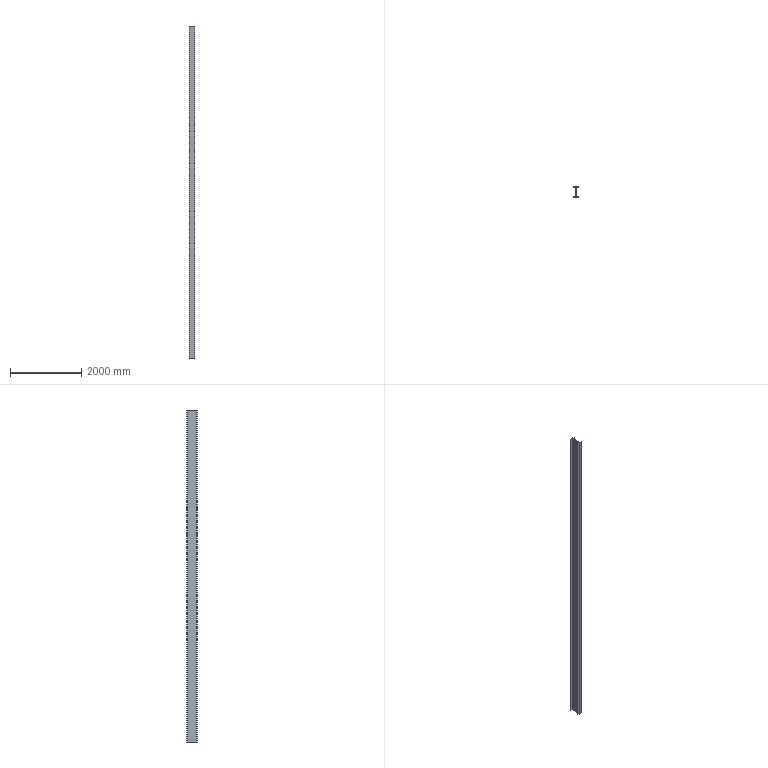Part | SolidWorks | features Extrusion 1 | 1 solid | 18 faces | box 150 x 300 x 9347 mm | volume 43725928 mm3 | plane 14 | cylinder 4 | commonest cylinder face diameters 26 x4
STEP:
#1=CARTESIAN_POINT('',(-75.,9.,0.));
#2=VERTEX_POINT('',#1);
#3=CARTESIAN_POINT('',(-75.,0.,0.));
#4=VERTEX_POINT('',#3);
#5=CARTESIAN_POINT('',(-75.,0.,0.));
#6=DIRECTION('',(0.,-1.,0.));
#7=VECTOR('',#6,1000.);
#8=LINE('',#5,#7);
#9=EDGE_CURVE('',#2,#4,#8,.T.);
#10=ORIENTED_EDGE('',*,*,#9,.T.);
#11=CARTESIAN_POINT('',(-75.,0.,9347.));
#12=VERTEX_POINT('',#11);
#13=CARTESIAN_POINT('',(-75.,0.,9347.));
#14=DIRECTION('',(0.,0.,-1.));
#15=VECTOR('',#14,1000.);
#16=LINE('',#13,#15);
#17=EDGE_CURVE('',#12,#4,#16,.T.);
#18=ORIENTED_EDGE('',*,*,#17,.F.);
#19=CARTESIAN_POINT('',(-75.,9.,9347.));
#20=VERTEX_POINT('',#19);
#21=CARTESIAN_POINT('',(-75.,0.,9347.));
#22=DIRECTION('',(0.,-1.,0.));
#23=VECTOR('',#22,1000.);
#24=LINE('',#21,#23);
#25=EDGE_CURVE('',#20,#12,#24,.T.);
#26=ORIENTED_EDGE('',*,*,#25,.F.);
#27=CARTESIAN_POINT('',(-75.,9.,9347.));
#28=DIRECTION('',(0.,0.,-1.));
#29=VECTOR('',#28,1000.);
#30=LINE('',#27,#29);
#31=EDGE_CURVE('',#20,#2,#30,.T.);
#32=ORIENTED_EDGE('',*,*,#31,.T.);
#33=EDGE_LOOP('',(#10,#18,#26,#32));
#34=FACE_OUTER_BOUND('',#33,.T.);
#35=CARTESIAN_POINT('',(-75.,0.,9347.));
#36=DIRECTION('',(1.,0.,0.));
#37=DIRECTION('',(0.,0.,-1.));
#38=AXIS2_PLACEMENT_3D('',#35,#36,#37);
#39=PLANE('',#38);
#40=ADVANCED_FACE('',(#34),#39,.F.);
#41=CARTESIAN_POINT('',(75.,0.,0.));
#42=VERTEX_POINT('',#41);
#43=CARTESIAN_POINT('',(75.,0.,0.));
#44=DIRECTION('',(1.,0.,0.));
#45=VECTOR('',#44,1000.);
#46=LINE('',#43,#45);
#47=EDGE_CURVE('',#4,#42,#46,.T.);
#48=ORIENTED_EDGE('',*,*,#47,.T.);
#49=CARTESIAN_POINT('',(75.,0.,9347.));
#50=VERTEX_POINT('',#49);
#51=CARTESIAN_POINT('',(75.,0.,9347.));
#52=DIRECTION('',(0.,0.,-1.));
#53=VECTOR('',#52,1000.);
#54=LINE('',#51,#53);
#55=EDGE_CURVE('',#50,#42,#54,.T.);
#56=ORIENTED_EDGE('',*,*,#55,.F.);
#57=CARTESIAN_POINT('',(75.,0.,9347.));
#58=DIRECTION('',(1.,0.,0.));
#59=VECTOR('',#58,1000.);
#60=LINE('',#57,#59);
#61=EDGE_CURVE('',#12,#50,#60,.T.);
#62=ORIENTED_EDGE('',*,*,#61,.F.);
#63=ORIENTED_EDGE('',*,*,#17,.T.);
#64=EDGE_LOOP('',(#48,#56,#62,#63));
#65=FACE_OUTER_BOUND('',#64,.T.);
#66=CARTESIAN_POINT('',(75.,0.,9347.));
#67=DIRECTION('',(0.,1.,0.));
#68=DIRECTION('',(-1.,0.,0.));
#69=AXIS2_PLACEMENT_3D('',#66,#67,#68);
#70=PLANE('',#69);
#71=ADVANCED_FACE('',(#65),#70,.F.);
#72=CARTESIAN_POINT('',(75.,9.,0.));
#73=VERTEX_POINT('',#72);
#74=CARTESIAN_POINT('',(75.,0.,0.));
#75=DIRECTION('',(0.,1.,0.));
#76=VECTOR('',#75,1000.);
#77=LINE('',#74,#76);
#78=EDGE_CURVE('',#42,#73,#77,.T.);
#79=ORIENTED_EDGE('',*,*,#78,.T.);
#80=CARTESIAN_POINT('',(75.,9.,9347.));
#81=VERTEX_POINT('',#80);
#82=CARTESIAN_POINT('',(75.,9.,9347.));
#83=DIRECTION('',(0.,0.,-1.));
#84=VECTOR('',#83,1000.);
#85=LINE('',#82,#84);
#86=EDGE_CURVE('',#81,#73,#85,.T.);
#87=ORIENTED_EDGE('',*,*,#86,.F.);
#88=CARTESIAN_POINT('',(75.,0.,9347.));
#89=DIRECTION('',(0.,1.,0.));
#90=VECTOR('',#89,1000.);
#91=LINE('',#88,#90);
#92=EDGE_CURVE('',#50,#81,#91,.T.);
#93=ORIENTED_EDGE('',*,*,#92,.F.);
#94=ORIENTED_EDGE('',*,*,#55,.T.);
#95=EDGE_LOOP('',(#79,#87,#93,#94));
#96=FACE_OUTER_BOUND('',#95,.T.);
#97=CARTESIAN_POINT('',(75.,0.,9347.));
#98=DIRECTION('',(-1.,0.,0.));
#99=DIRECTION('',(0.,0.,1.));
#100=AXIS2_PLACEMENT_3D('',#97,#98,#99);
#101=PLANE('',#100);
#102=ADVANCED_FACE('',(#96),#101,.F.);
#103=CARTESIAN_POINT('',(16.25,9.,0.));
#104=VERTEX_POINT('',#103);
#105=CARTESIAN_POINT('',(75.,9.,0.));
#106=DIRECTION('',(-1.,0.,0.));
#107=VECTOR('',#106,1000.);
#108=LINE('',#105,#107);
#109=EDGE_CURVE('',#73,#104,#108,.T.);
#110=ORIENTED_EDGE('',*,*,#109,.T.);
#111=CARTESIAN_POINT('',(16.25,9.,9347.));
#112=VERTEX_POINT('',#111);
#113=CARTESIAN_POINT('',(16.25,9.,9347.));
#114=DIRECTION('',(0.,0.,-1.));
#115=VECTOR('',#114,1000.);
#116=LINE('',#113,#115);
#117=EDGE_CURVE('',#112,#104,#116,.T.);
#118=ORIENTED_EDGE('',*,*,#117,.F.);
#119=CARTESIAN_POINT('',(75.,9.,9347.));
#120=DIRECTION('',(-1.,0.,0.));
#121=VECTOR('',#120,1000.);
#122=LINE('',#119,#121);
#123=EDGE_CURVE('',#81,#112,#122,.T.);
#124=ORIENTED_EDGE('',*,*,#123,.F.);
#125=ORIENTED_EDGE('',*,*,#86,.T.);
#126=EDGE_LOOP('',(#110,#118,#124,#125));
#127=FACE_OUTER_BOUND('',#126,.T.);
#128=CARTESIAN_POINT('',(75.,9.,9347.));
#129=DIRECTION('',(0.,-1.,0.));
#130=DIRECTION('',(1.,0.,0.));
#131=AXIS2_PLACEMENT_3D('',#128,#129,#130);
#132=PLANE('',#131);
#133=ADVANCED_FACE('',(#127),#132,.F.);
#134=CARTESIAN_POINT('',(3.25,22.,0.));
#135=VERTEX_POINT('',#134);
#136=CARTESIAN_POINT('',(16.25,22.,0.));
#137=DIRECTION('',(0.,0.,-1.));
#138=DIRECTION('',(-1.,0.,0.));
#139=AXIS2_PLACEMENT_3D('',#136,#137,#138);
#140=CIRCLE('',#139,13.);
#141=EDGE_CURVE('',#104,#135,#140,.T.);
#142=ORIENTED_EDGE('',*,*,#141,.T.);
#143=CARTESIAN_POINT('',(3.25,22.,9347.));
#144=VERTEX_POINT('',#143);
#145=CARTESIAN_POINT('',(3.25,22.,9347.));
#146=DIRECTION('',(0.,0.,-1.));
#147=VECTOR('',#146,1000.);
#148=LINE('',#145,#147);
#149=EDGE_CURVE('',#144,#135,#148,.T.);
#150=ORIENTED_EDGE('',*,*,#149,.F.);
#151=CARTESIAN_POINT('',(16.25,22.,9347.));
#152=DIRECTION('',(0.,0.,-1.));
#153=DIRECTION('',(-1.,0.,0.));
#154=AXIS2_PLACEMENT_3D('',#151,#152,#153);
#155=CIRCLE('',#154,13.);
#156=EDGE_CURVE('',#112,#144,#155,.T.);
#157=ORIENTED_EDGE('',*,*,#156,.F.);
#158=ORIENTED_EDGE('',*,*,#117,.T.);
#159=EDGE_LOOP('',(#142,#150,#157,#158));
#160=FACE_OUTER_BOUND('',#159,.T.);
#161=CARTESIAN_POINT('',(16.25,22.,9347.));
#162=DIRECTION('',(0.,0.,-1.));
#163=DIRECTION('',(-1.,0.,0.));
#164=AXIS2_PLACEMENT_3D('',#161,#162,#163);
#165=CYLINDRICAL_SURFACE('',#164,13.);
#166=ADVANCED_FACE('',(#160),#165,.F.);
#167=CARTESIAN_POINT('',(3.25,278.,0.));
#168=VERTEX_POINT('',#167);
#169=CARTESIAN_POINT('',(3.25,22.,0.));
#170=DIRECTION('',(0.,1.,0.));
#171=VECTOR('',#170,1000.);
#172=LINE('',#169,#171);
#173=EDGE_CURVE('',#135,#168,#172,.T.);
#174=ORIENTED_EDGE('',*,*,#173,.T.);
#175=CARTESIAN_POINT('',(3.25,278.,9347.));
#176=VERTEX_POINT('',#175);
#177=CARTESIAN_POINT('',(3.25,278.,9347.));
#178=DIRECTION('',(0.,0.,-1.));
#179=VECTOR('',#178,1000.);
#180=LINE('',#177,#179);
#181=EDGE_CURVE('',#176,#168,#180,.T.);
#182=ORIENTED_EDGE('',*,*,#181,.F.);
#183=CARTESIAN_POINT('',(3.25,22.,9347.));
#184=DIRECTION('',(0.,1.,0.));
#185=VECTOR('',#184,1000.);
#186=LINE('',#183,#185);
#187=EDGE_CURVE('',#144,#176,#186,.T.);
#188=ORIENTED_EDGE('',*,*,#187,.F.);
#189=ORIENTED_EDGE('',*,*,#149,.T.);
#190=EDGE_LOOP('',(#174,#182,#188,#189));
#191=FACE_OUTER_BOUND('',#190,.T.);
#192=CARTESIAN_POINT('',(3.25,22.,9347.));
#193=DIRECTION('',(-1.,0.,0.));
#194=DIRECTION('',(0.,0.,1.));
#195=AXIS2_PLACEMENT_3D('',#192,#193,#194);
#196=PLANE('',#195);
#197=ADVANCED_FACE('',(#191),#196,.F.);
#198=CARTESIAN_POINT('',(16.25,291.,0.));
#199=VERTEX_POINT('',#198);
#200=CARTESIAN_POINT('',(16.25,278.,0.));
#201=DIRECTION('',(0.,0.,-1.));
#202=DIRECTION('',(-1.,0.,0.));
#203=AXIS2_PLACEMENT_3D('',#200,#201,#202);
#204=CIRCLE('',#203,13.);
#205=EDGE_CURVE('',#168,#199,#204,.T.);
#206=ORIENTED_EDGE('',*,*,#205,.T.);
#207=CARTESIAN_POINT('',(16.25,291.,9347.));
#208=VERTEX_POINT('',#207);
#209=CARTESIAN_POINT('',(16.25,291.,9347.));
#210=DIRECTION('',(0.,0.,-1.));
#211=VECTOR('',#210,1000.);
#212=LINE('',#209,#211);
#213=EDGE_CURVE('',#208,#199,#212,.T.);
#214=ORIENTED_EDGE('',*,*,#213,.F.);
#215=CARTESIAN_POINT('',(16.25,278.,9347.));
#216=DIRECTION('',(0.,0.,-1.));
#217=DIRECTION('',(-1.,0.,0.));
#218=AXIS2_PLACEMENT_3D('',#215,#216,#217);
#219=CIRCLE('',#218,13.);
#220=EDGE_CURVE('',#176,#208,#219,.T.);
#221=ORIENTED_EDGE('',*,*,#220,.F.);
#222=ORIENTED_EDGE('',*,*,#181,.T.);
#223=EDGE_LOOP('',(#206,#214,#221,#222));
#224=FACE_OUTER_BOUND('',#223,.T.);
#225=CARTESIAN_POINT('',(16.25,278.,9347.));
#226=DIRECTION('',(0.,0.,-1.));
#227=DIRECTION('',(-1.,0.,0.));
#228=AXIS2_PLACEMENT_3D('',#225,#226,#227);
#229=CYLINDRICAL_SURFACE('',#228,13.);
#230=ADVANCED_FACE('',(#224),#229,.F.);
#231=CARTESIAN_POINT('',(75.,291.,0.));
#232=VERTEX_POINT('',#231);
#233=CARTESIAN_POINT('',(16.25,291.,0.));
#234=DIRECTION('',(1.,0.,0.));
#235=VECTOR('',#234,1000.);
#236=LINE('',#233,#235);
#237=EDGE_CURVE('',#199,#232,#236,.T.);
#238=ORIENTED_EDGE('',*,*,#237,.T.);
#239=CARTESIAN_POINT('',(75.,291.,9347.));
#240=VERTEX_POINT('',#239);
#241=CARTESIAN_POINT('',(75.,291.,9347.));
#242=DIRECTION('',(0.,0.,-1.));
#243=VECTOR('',#242,1000.);
#244=LINE('',#241,#243);
#245=EDGE_CURVE('',#240,#232,#244,.T.);
#246=ORIENTED_EDGE('',*,*,#245,.F.);
#247=CARTESIAN_POINT('',(16.25,291.,9347.));
#248=DIRECTION('',(1.,0.,0.));
#249=VECTOR('',#248,1000.);
#250=LINE('',#247,#249);
#251=EDGE_CURVE('',#208,#240,#250,.T.);
#252=ORIENTED_EDGE('',*,*,#251,.F.);
#253=ORIENTED_EDGE('',*,*,#213,.T.);
#254=EDGE_LOOP('',(#238,#246,#252,#253));
#255=FACE_OUTER_BOUND('',#254,.T.);
#256=CARTESIAN_POINT('',(16.25,291.,9347.));
#257=DIRECTION('',(0.,1.,0.));
#258=DIRECTION('',(-1.,0.,0.));
#259=AXIS2_PLACEMENT_3D('',#256,#257,#258);
#260=PLANE('',#259);
#261=ADVANCED_FACE('',(#255),#260,.F.);
#262=CARTESIAN_POINT('',(75.,300.,0.));
#263=VERTEX_POINT('',#262);
#264=CARTESIAN_POINT('',(75.,291.,0.));
#265=DIRECTION('',(0.,1.,0.));
#266=VECTOR('',#265,1000.);
#267=LINE('',#264,#266);
#268=EDGE_CURVE('',#232,#263,#267,.T.);
#269=ORIENTED_EDGE('',*,*,#268,.T.);
#270=CARTESIAN_POINT('',(75.,300.,9347.));
#271=VERTEX_POINT('',#270);
#272=CARTESIAN_POINT('',(75.,300.,9347.));
#273=DIRECTION('',(0.,0.,-1.));
#274=VECTOR('',#273,1000.);
#275=LINE('',#272,#274);
#276=EDGE_CURVE('',#271,#263,#275,.T.);
#277=ORIENTED_EDGE('',*,*,#276,.F.);
#278=CARTESIAN_POINT('',(75.,291.,9347.));
#279=DIRECTION('',(0.,1.,0.));
#280=VECTOR('',#279,1000.);
#281=LINE('',#278,#280);
#282=EDGE_CURVE('',#240,#271,#281,.T.);
#283=ORIENTED_EDGE('',*,*,#282,.F.);
#284=ORIENTED_EDGE('',*,*,#245,.T.);
#285=EDGE_LOOP('',(#269,#277,#283,#284));
#286=FACE_OUTER_BOUND('',#285,.T.);
#287=CARTESIAN_POINT('',(75.,291.,9347.));
#288=DIRECTION('',(-1.,0.,0.));
#289=DIRECTION('',(0.,-1.,0.));
#290=AXIS2_PLACEMENT_3D('',#287,#288,#289);
#291=PLANE('',#290);
#292=ADVANCED_FACE('',(#286),#291,.F.);
#293=CARTESIAN_POINT('',(-75.,300.,0.));
#294=VERTEX_POINT('',#293);
#295=CARTESIAN_POINT('',(-75.,300.,0.));
#296=DIRECTION('',(-1.,0.,0.));
#297=VECTOR('',#296,1000.);
#298=LINE('',#295,#297);
#299=EDGE_CURVE('',#263,#294,#298,.T.);
#300=ORIENTED_EDGE('',*,*,#299,.T.);
#301=CARTESIAN_POINT('',(-75.,300.,9347.));
#302=VERTEX_POINT('',#301);
#303=CARTESIAN_POINT('',(-75.,300.,9347.));
#304=DIRECTION('',(0.,0.,-1.));
#305=VECTOR('',#304,1000.);
#306=LINE('',#303,#305);
#307=EDGE_CURVE('',#302,#294,#306,.T.);
#308=ORIENTED_EDGE('',*,*,#307,.F.);
#309=CARTESIAN_POINT('',(-75.,300.,9347.));
#310=DIRECTION('',(-1.,0.,0.));
#311=VECTOR('',#310,1000.);
#312=LINE('',#309,#311);
#313=EDGE_CURVE('',#271,#302,#312,.T.);
#314=ORIENTED_EDGE('',*,*,#313,.F.);
#315=ORIENTED_EDGE('',*,*,#276,.T.);
#316=EDGE_LOOP('',(#300,#308,#314,#315));
#317=FACE_OUTER_BOUND('',#316,.T.);
#318=CARTESIAN_POINT('',(-75.,300.,9347.));
#319=DIRECTION('',(0.,-1.,0.));
#320=DIRECTION('',(0.,0.,-1.));
#321=AXIS2_PLACEMENT_3D('',#318,#319,#320);
#322=PLANE('',#321);
#323=ADVANCED_FACE('',(#317),#322,.F.);
#324=CARTESIAN_POINT('',(-75.,291.,0.));
#325=VERTEX_POINT('',#324);
#326=CARTESIAN_POINT('',(-75.,291.,0.));
#327=DIRECTION('',(0.,-1.,0.));
#328=VECTOR('',#327,1000.);
#329=LINE('',#326,#328);
#330=EDGE_CURVE('',#294,#325,#329,.T.);
#331=ORIENTED_EDGE('',*,*,#330,.T.);
#332=CARTESIAN_POINT('',(-75.,291.,9347.));
#333=VERTEX_POINT('',#332);
#334=CARTESIAN_POINT('',(-75.,291.,9347.));
#335=DIRECTION('',(0.,0.,-1.));
#336=VECTOR('',#335,1000.);
#337=LINE('',#334,#336);
#338=EDGE_CURVE('',#333,#325,#337,.T.);
#339=ORIENTED_EDGE('',*,*,#338,.F.);
#340=CARTESIAN_POINT('',(-75.,291.,9347.));
#341=DIRECTION('',(0.,-1.,0.));
#342=VECTOR('',#341,1000.);
#343=LINE('',#340,#342);
#344=EDGE_CURVE('',#302,#333,#343,.T.);
#345=ORIENTED_EDGE('',*,*,#344,.F.);
#346=ORIENTED_EDGE('',*,*,#307,.T.);
#347=EDGE_LOOP('',(#331,#339,#345,#346));
#348=FACE_OUTER_BOUND('',#347,.T.);
#349=CARTESIAN_POINT('',(-75.,291.,9347.));
#350=DIRECTION('',(1.,0.,0.));
#351=DIRECTION('',(0.,1.,0.));
#352=AXIS2_PLACEMENT_3D('',#349,#350,#351);
#353=PLANE('',#352);
#354=ADVANCED_FACE('',(#348),#353,.F.);
#355=CARTESIAN_POINT('',(-16.25,291.,0.));
#356=VERTEX_POINT('',#355);
#357=CARTESIAN_POINT('',(-16.25,291.,0.));
#358=DIRECTION('',(1.,0.,0.));
#359=VECTOR('',#358,1000.);
#360=LINE('',#357,#359);
#361=EDGE_CURVE('',#325,#356,#360,.T.);
#362=ORIENTED_EDGE('',*,*,#361,.T.);
#363=CARTESIAN_POINT('',(-16.25,291.,9347.));
#364=VERTEX_POINT('',#363);
#365=CARTESIAN_POINT('',(-16.25,291.,9347.));
#366=DIRECTION('',(0.,0.,-1.));
#367=VECTOR('',#366,1000.);
#368=LINE('',#365,#367);
#369=EDGE_CURVE('',#364,#356,#368,.T.);
#370=ORIENTED_EDGE('',*,*,#369,.F.);
#371=CARTESIAN_POINT('',(-16.25,291.,9347.));
#372=DIRECTION('',(1.,0.,0.));
#373=VECTOR('',#372,1000.);
#374=LINE('',#371,#373);
#375=EDGE_CURVE('',#333,#364,#374,.T.);
#376=ORIENTED_EDGE('',*,*,#375,.F.);
#377=ORIENTED_EDGE('',*,*,#338,.T.);
#378=EDGE_LOOP('',(#362,#370,#376,#377));
#379=FACE_OUTER_BOUND('',#378,.T.);
#380=CARTESIAN_POINT('',(-16.25,291.,9347.));
#381=DIRECTION('',(0.,1.,0.));
#382=DIRECTION('',(-1.,0.,0.));
#383=AXIS2_PLACEMENT_3D('',#380,#381,#382);
#384=PLANE('',#383);
#385=ADVANCED_FACE('',(#379),#384,.F.);
#386=CARTESIAN_POINT('',(-3.25,278.,0.));
#387=VERTEX_POINT('',#386);
#388=CARTESIAN_POINT('',(-16.25,278.,0.));
#389=DIRECTION('',(0.,0.,-1.));
#390=DIRECTION('',(1.,0.,0.));
#391=AXIS2_PLACEMENT_3D('',#388,#389,#390);
#392=CIRCLE('',#391,13.);
#393=EDGE_CURVE('',#356,#387,#392,.T.);
#394=ORIENTED_EDGE('',*,*,#393,.T.);
#395=CARTESIAN_POINT('',(-3.25,278.,9347.));
#396=VERTEX_POINT('',#395);
#397=CARTESIAN_POINT('',(-3.25,278.,9347.));
#398=DIRECTION('',(0.,0.,-1.));
#399=VECTOR('',#398,1000.);
#400=LINE('',#397,#399);
#401=EDGE_CURVE('',#396,#387,#400,.T.);
#402=ORIENTED_EDGE('',*,*,#401,.F.);
#403=CARTESIAN_POINT('',(-16.25,278.,9347.));
#404=DIRECTION('',(0.,0.,-1.));
#405=DIRECTION('',(1.,0.,0.));
#406=AXIS2_PLACEMENT_3D('',#403,#404,#405);
#407=CIRCLE('',#406,13.);
#408=EDGE_CURVE('',#364,#396,#407,.T.);
#409=ORIENTED_EDGE('',*,*,#408,.F.);
#410=ORIENTED_EDGE('',*,*,#369,.T.);
#411=EDGE_LOOP('',(#394,#402,#409,#410));
#412=FACE_OUTER_BOUND('',#411,.T.);
#413=CARTESIAN_POINT('',(-16.25,278.,9347.));
#414=DIRECTION('',(0.,0.,-1.));
#415=DIRECTION('',(-1.,0.,0.));
#416=AXIS2_PLACEMENT_3D('',#413,#414,#415);
#417=CYLINDRICAL_SURFACE('',#416,13.);
#418=ADVANCED_FACE('',(#412),#417,.F.);
#419=CARTESIAN_POINT('',(-3.25,22.,0.));
#420=VERTEX_POINT('',#419);
#421=CARTESIAN_POINT('',(-3.25,22.,0.));
#422=DIRECTION('',(0.,-1.,0.));
#423=VECTOR('',#422,1000.);
#424=LINE('',#421,#423);
#425=EDGE_CURVE('',#387,#420,#424,.T.);
#426=ORIENTED_EDGE('',*,*,#425,.T.);
#427=CARTESIAN_POINT('',(-3.25,22.,9347.));
#428=VERTEX_POINT('',#427);
#429=CARTESIAN_POINT('',(-3.25,22.,9347.));
#430=DIRECTION('',(0.,0.,-1.));
#431=VECTOR('',#430,1000.);
#432=LINE('',#429,#431);
#433=EDGE_CURVE('',#428,#420,#432,.T.);
#434=ORIENTED_EDGE('',*,*,#433,.F.);
#435=CARTESIAN_POINT('',(-3.25,22.,9347.));
#436=DIRECTION('',(0.,-1.,0.));
#437=VECTOR('',#436,1000.);
#438=LINE('',#435,#437);
#439=EDGE_CURVE('',#396,#428,#438,.T.);
#440=ORIENTED_EDGE('',*,*,#439,.F.);
#441=ORIENTED_EDGE('',*,*,#401,.T.);
#442=EDGE_LOOP('',(#426,#434,#440,#441));
#443=FACE_OUTER_BOUND('',#442,.T.);
#444=CARTESIAN_POINT('',(-3.25,22.,9347.));
#445=DIRECTION('',(1.,0.,0.));
#446=DIRECTION('',(0.,0.,-1.));
#447=AXIS2_PLACEMENT_3D('',#444,#445,#446);
#448=PLANE('',#447);
#449=ADVANCED_FACE('',(#443),#448,.F.);
#450=CARTESIAN_POINT('',(-16.25,9.,0.));
#451=VERTEX_POINT('',#450);
#452=CARTESIAN_POINT('',(-16.25,22.,0.));
#453=DIRECTION('',(0.,0.,-1.));
#454=DIRECTION('',(-1.,0.,0.));
#455=AXIS2_PLACEMENT_3D('',#452,#453,#454);
#456=CIRCLE('',#455,13.);
#457=EDGE_CURVE('',#420,#451,#456,.T.);
#458=ORIENTED_EDGE('',*,*,#457,.T.);
#459=CARTESIAN_POINT('',(-16.25,9.,9347.));
#460=VERTEX_POINT('',#459);
#461=CARTESIAN_POINT('',(-16.25,9.,9347.));
#462=DIRECTION('',(0.,0.,-1.));
#463=VECTOR('',#462,1000.);
#464=LINE('',#461,#463);
#465=EDGE_CURVE('',#460,#451,#464,.T.);
#466=ORIENTED_EDGE('',*,*,#465,.F.);
#467=CARTESIAN_POINT('',(-16.25,22.,9347.));
#468=DIRECTION('',(0.,0.,-1.));
#469=DIRECTION('',(-1.,0.,0.));
#470=AXIS2_PLACEMENT_3D('',#467,#468,#469);
#471=CIRCLE('',#470,13.);
#472=EDGE_CURVE('',#428,#460,#471,.T.);
#473=ORIENTED_EDGE('',*,*,#472,.F.);
#474=ORIENTED_EDGE('',*,*,#433,.T.);
#475=EDGE_LOOP('',(#458,#466,#473,#474));
#476=FACE_OUTER_BOUND('',#475,.T.);
#477=CARTESIAN_POINT('',(-16.25,22.,9347.));
#478=DIRECTION('',(0.,0.,-1.));
#479=DIRECTION('',(-1.,0.,0.));
#480=AXIS2_PLACEMENT_3D('',#477,#478,#479);
#481=CYLINDRICAL_SURFACE('',#480,13.);
#482=ADVANCED_FACE('',(#476),#481,.F.);
#483=CARTESIAN_POINT('',(-75.,9.,0.));
#484=DIRECTION('',(-1.,0.,0.));
#485=VECTOR('',#484,1000.);
#486=LINE('',#483,#485);
#487=EDGE_CURVE('',#451,#2,#486,.T.);
#488=ORIENTED_EDGE('',*,*,#487,.T.);
#489=ORIENTED_EDGE('',*,*,#31,.F.);
#490=CARTESIAN_POINT('',(-75.,9.,9347.));
#491=DIRECTION('',(-1.,0.,0.));
#492=VECTOR('',#491,1000.);
#493=LINE('',#490,#492);
#494=EDGE_CURVE('',#460,#20,#493,.T.);
#495=ORIENTED_EDGE('',*,*,#494,.F.);
#496=ORIENTED_EDGE('',*,*,#465,.T.);
#497=EDGE_LOOP('',(#488,#489,#495,#496));
#498=FACE_OUTER_BOUND('',#497,.T.);
#499=CARTESIAN_POINT('',(-75.,9.,9347.));
#500=DIRECTION('',(0.,-1.,0.));
#501=DIRECTION('',(1.,0.,0.));
#502=AXIS2_PLACEMENT_3D('',#499,#500,#501);
#503=PLANE('',#502);
#504=ADVANCED_FACE('',(#498),#503,.F.);
#505=ORIENTED_EDGE('',*,*,#25,.T.);
#506=ORIENTED_EDGE('',*,*,#61,.T.);
#507=ORIENTED_EDGE('',*,*,#92,.T.);
#508=ORIENTED_EDGE('',*,*,#123,.T.);
#509=ORIENTED_EDGE('',*,*,#156,.T.);
#510=ORIENTED_EDGE('',*,*,#187,.T.);
#511=ORIENTED_EDGE('',*,*,#220,.T.);
#512=ORIENTED_EDGE('',*,*,#251,.T.);
#513=ORIENTED_EDGE('',*,*,#282,.T.);
#514=ORIENTED_EDGE('',*,*,#313,.T.);
#515=ORIENTED_EDGE('',*,*,#344,.T.);
#516=ORIENTED_EDGE('',*,*,#375,.T.);
#517=ORIENTED_EDGE('',*,*,#408,.T.);
#518=ORIENTED_EDGE('',*,*,#439,.T.);
#519=ORIENTED_EDGE('',*,*,#472,.T.);
#520=ORIENTED_EDGE('',*,*,#494,.T.);
#521=EDGE_LOOP('',(#505,#506,#507,#508,#509,#510,#511,#512,#513,#514,#515,#516,#517,#518,#519,#520));
#522=FACE_OUTER_BOUND('',#521,.T.);
#523=CARTESIAN_POINT('',(-16.25,22.,9347.));
#524=DIRECTION('',(0.,0.,-1.));
#525=DIRECTION('',(-1.,0.,0.));
#526=AXIS2_PLACEMENT_3D('',#523,#524,#525);
#527=PLANE('',#526);
#528=ADVANCED_FACE('',(#522),#527,.F.);
#529=ORIENTED_EDGE('',*,*,#9,.F.);
#530=ORIENTED_EDGE('',*,*,#487,.F.);
#531=ORIENTED_EDGE('',*,*,#457,.F.);
#532=ORIENTED_EDGE('',*,*,#425,.F.);
#533=ORIENTED_EDGE('',*,*,#393,.F.);
#534=ORIENTED_EDGE('',*,*,#361,.F.);
#535=ORIENTED_EDGE('',*,*,#330,.F.);
#536=ORIENTED_EDGE('',*,*,#299,.F.);
#537=ORIENTED_EDGE('',*,*,#268,.F.);
#538=ORIENTED_EDGE('',*,*,#237,.F.);
#539=ORIENTED_EDGE('',*,*,#205,.F.);
#540=ORIENTED_EDGE('',*,*,#173,.F.);
#541=ORIENTED_EDGE('',*,*,#141,.F.);
#542=ORIENTED_EDGE('',*,*,#109,.F.);
#543=ORIENTED_EDGE('',*,*,#78,.F.);
#544=ORIENTED_EDGE('',*,*,#47,.F.);
#545=EDGE_LOOP('',(#529,#530,#531,#532,#533,#534,#535,#536,#537,#538,#539,#540,#541,#542,#543,#544));
#546=FACE_OUTER_BOUND('',#545,.T.);
#547=CARTESIAN_POINT('',(-16.25,22.,0.));
#548=DIRECTION('',(0.,0.,-1.));
#549=DIRECTION('',(-1.,0.,0.));
#550=AXIS2_PLACEMENT_3D('',#547,#548,#549);
#551=PLANE('',#550);
#552=ADVANCED_FACE('',(#546),#551,.T.);
#553=CLOSED_SHELL('',(#40,#71,#102,#133,#166,#197,#230,#261,#292,#323,#354,#385,#418,#449,#482,#504,#528,#552));
#554=MANIFOLD_SOLID_BREP('',#553);
#555=CARTESIAN_POINT('',(0.,0.,0.));
#556=DIRECTION('',(0.,0.,1.));
#557=DIRECTION('',(1.,0.,0.));
#558=AXIS2_PLACEMENT_3D('',#555,#556,#557);
#559=(LENGTH_UNIT()NAMED_UNIT(*)SI_UNIT(.MILLI.,.METRE.));
#560=UNCERTAINTY_MEASURE_WITH_UNIT(LENGTH_MEASURE(0.00001),#559,'','');
#561=(NAMED_UNIT(*)PLANE_ANGLE_UNIT()SI_UNIT($,.RADIAN.));
#562=(NAMED_UNIT(*)SI_UNIT($,.STERADIAN.)SOLID_ANGLE_UNIT());
#563=(GEOMETRIC_REPRESENTATION_CONTEXT(3)GLOBAL_UNCERTAINTY_ASSIGNED_CONTEXT((#560))GLOBAL_UNIT_ASSIGNED_CONTEXT((#559,#561,#562))REPRESENTATION_CONTEXT('',''));
#564=ADVANCED_BREP_SHAPE_REPRESENTATION('',(#554,#558),#563);